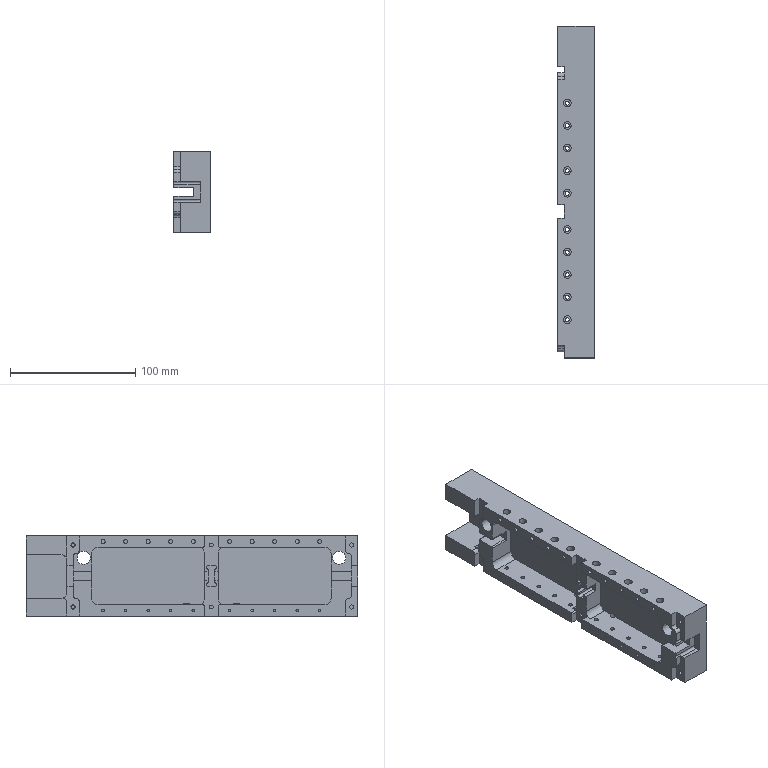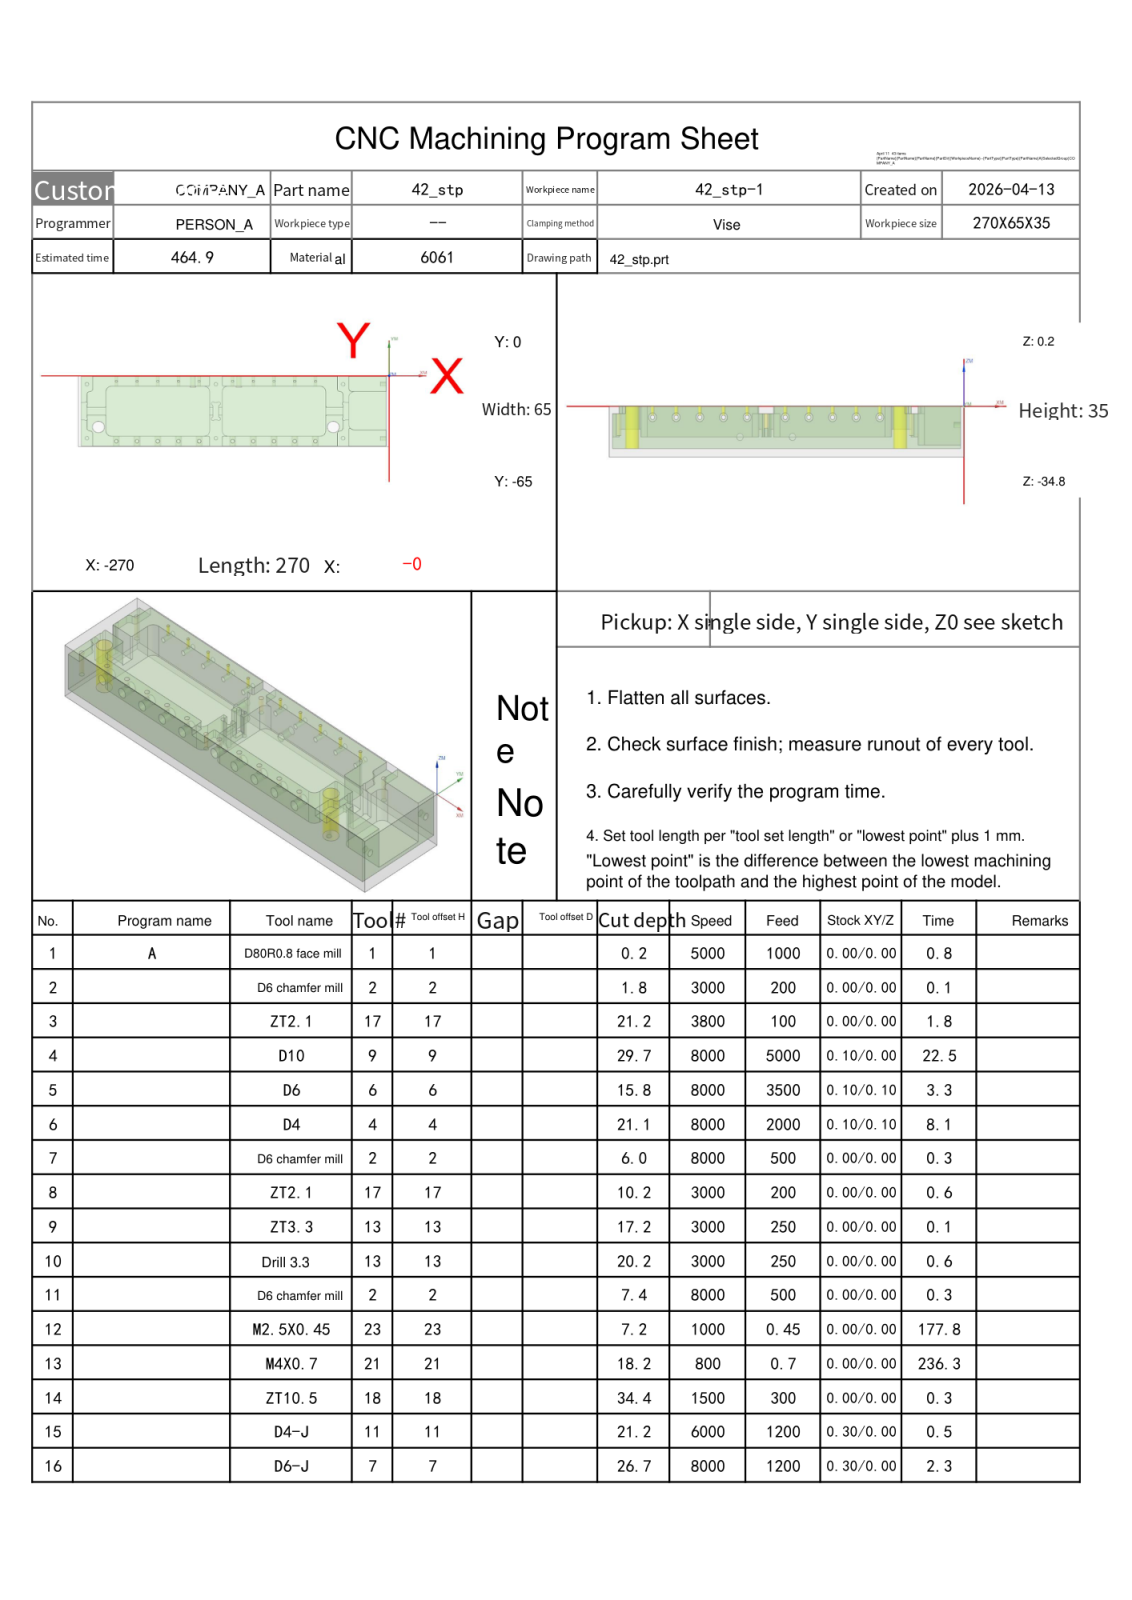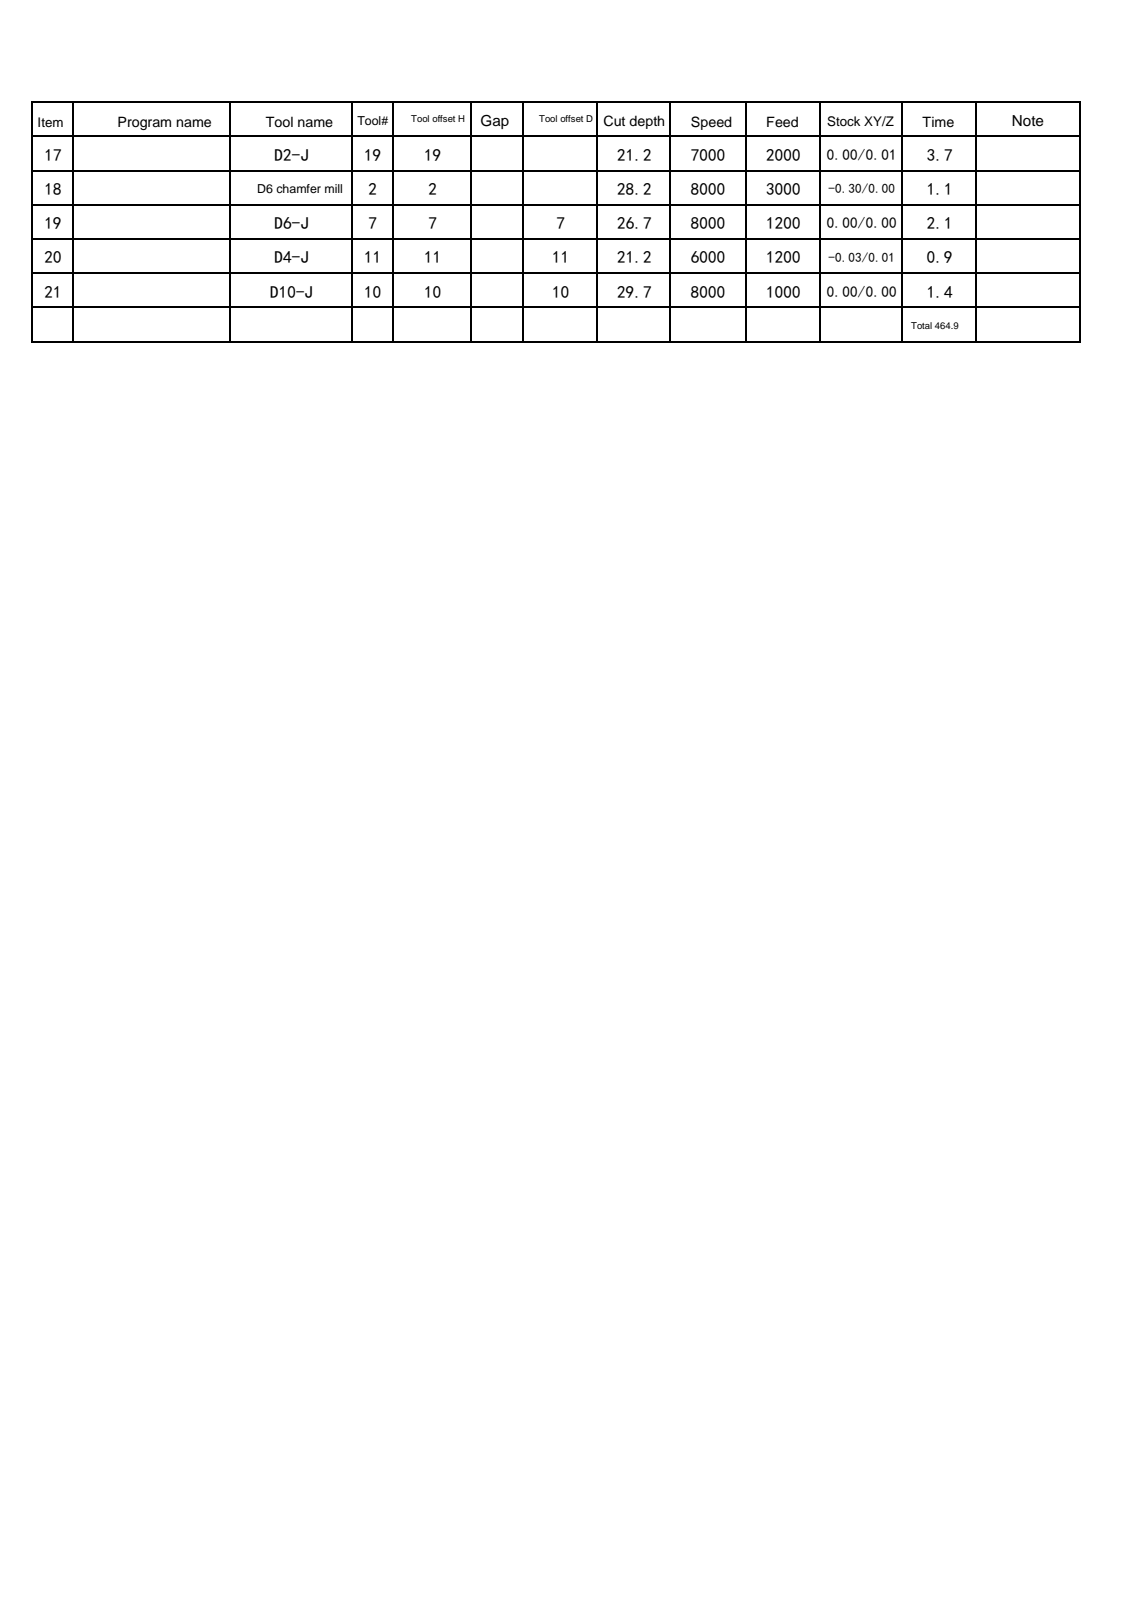NC program | NX | posted by the shop | part box 29 x 265 x 64 mm
Lines 1 to 4065 of 41846, first 2576 of 4063 lines:
%
O0001
(Machine time: 837.83 MIN)
(===Total Tool:14===)
(T1=D80R0.8 face mill D=80.  R=0.8  D-  H01 Z=-0.   )
(T2=D6 chamfer mill   D=6.   R=0.   D-  H02 Z=-28.  )
(T17=ZT2.1  D=2.1  DR_a=118 D-  H17 Z=-21.  )
(T9=D10     D=10.  R=0.   D-  H09 Z=-29.5 )
(T6=D6      D=6.   R=0.   D-  H06 Z=-15.6 )
(T4=D4      D=4.   R=0.   D-  H04 Z=-20.9 )
(T13=ZT3.3  D=3.3  DR_a=118 D-  H13 Z=-20.  )
(T23=M2.5X0.45 D=2.05 DR_a=180 D-  H23 Z=-7.   )
(T21=M4X0.7 D=3.3  DR_a=180 D-  H21 Z=-18.  )
(T18=ZT10.5 D=10.5 DR_a=118 D-  H18 Z=-34.15)
(T11=D4-J   D=4.   R=0.   D-  H11 Z=-21.  )
(T7=D6-J    D=6.   R=0.   D-  H07 Z=-26.5 )
(T19=D2-J   D=2.   R=0.   D-  H19 Z=-21.  )
(T10=D10-J  D=10.  R=0.   D10 H10 Z=-29.5 )
G80 G90 G17 G49 G40
G91 G28 Z0
M01
N1 T01 M06
(D80R0.8 face mill  D=80. R=0.8 H=01 ce=0.00 di=0.00)
G00 G90 G54 X-312.5 Y-8.5 M03 S5000
G43 H01 Z20.
M08
Z2.
G01 Z0.0 F1000.
X-307.5
X37.5
Y-56.5
X-307.5
X-312.5
Z2.
G00 Z20.
G91 G28 Z0.0
M05
M09
G91 G28 Z0.0
M01
N2 T02 M06
(D6 chamfer mill  D=6. R=0. H=02 ce=0.00 di=0.00)
G00 G90 G54 X-263.5 Y-25.5 M03 S3000
G43 H02 Z20.
M08
G98 G81 X-263.5 Y-25.5 Z-1.55 R1. F200.
Y-39.5
X-153. Y-25.5
Y-39.5
X-148. Y-25.5
Y-39.5
X-39. Y-25.5
Y-39.5
G80
G00 Z20.
G91 G28 Z0.0
M05
M09
G91 G28 Z0.0
M01
N3 T17 M06
(ZT2.1 D=2.1 DR_a=118 H=17)
G00 G90 G54 X-263.5 Y-25.5 M03 S3800
G43 H17 Z20.
M08
G98 G83 X-263.5 Y-25.5 Z-21. R1. F100. Q1.5
Y-39.5
X-153. Y-25.5
Y-39.5
X-148. Y-25.5
Y-39.5
X-39. Y-25.5
Y-39.5
G80
G00 Z20.
G91 G28 Z0.0
M05
M09
G91 G28 Z0.0
M01
N4 T09 M06
(D10  D=10. R=0. H=09 ce=0.10 di=0.00)
G00 G90 G54 X-135. Y-69.6 M03 S8000
G43 H09 Z20.
M08
Z.5
G01 X-267.5 Z.348 F5000.
G02 X-272.6 Y-64.5 Z.339 I0.0 J5.1
G01 Y-.5 Z.266
G02 X-267.5 Y4.6 Z.257 I5.1 J0.0
G01 X-2.5 Z-.046
G02 X2.6 Y-.5 Z-.055 I0.0 J-5.1
G01 Y-64.5 Z-.129
G02 X-2.5 Y-69.6 Z-.138 I-5.1 J0.0
G01 X-267.5 Z-.441
G02 X-272.6 Y-64.5 Z-.45 I0.0 J5.1
G01 Y-.5 Z-.523
G02 X-267.5 Y4.6 Z-.533 I5.1 J0.0
G01 X-2.5 Z-.836
G02 X2.6 Y-.5 Z-.845 I0.0 J-5.1
G01 Y-64.5 Z-.918
G02 X-2.5 Y-69.6 Z-.927 I-5.1 J0.0
G01 X-267.5 Z-1.231
G02 X-272.6 Y-64.5 Z-1.24 I0.0 J5.1
G01 Y-.5 Z-1.313
G02 X-267.5 Y4.6 Z-1.322 I5.1 J0.0
G01 X-2.5 Z-1.625
G02 X2.6 Y-.5 Z-1.634 I0.0 J-5.1
G01 Y-64.5 Z-1.708
G02 X-2.5 Y-69.6 Z-1.717 I-5.1 J0.0
G01 X-267.5 Z-2.02
G02 X-272.6 Y-64.5 Z-2.029 I0.0 J5.1
G01 Y-.5 Z-2.102
G02 X-267.5 Y4.6 Z-2.112 I5.1 J0.0
G01 X-2.5 Z-2.415
G02 X2.6 Y-.5 Z-2.424 I0.0 J-5.1
G01 Y-64.5 Z-2.497
G02 X-2.5 Y-69.6 Z-2.506 I-5.1 J0.0
G01 X-267.5 Z-2.809
G02 X-272.6 Y-64.5 Z-2.819 I0.0 J5.1
G01 Y-.5 Z-2.892
G02 X-267.5 Y4.6 Z-2.901 I5.1 J0.0
G01 X-2.5 Z-3.204
G02 X2.6 Y-.5 Z-3.213 I0.0 J-5.1
G01 Y-64.5 Z-3.287
G02 X-2.5 Y-69.6 Z-3.296 I-5.1 J0.0
G01 X-267.5 Z-3.599
G02 X-272.6 Y-64.5 Z-3.608 I0.0 J5.1
G01 Y-.5 Z-3.681
G02 X-267.5 Y4.6 Z-3.691 I5.1 J0.0
G01 X-2.5 Z-3.994
G02 X2.6 Y-.5 Z-4.003 I0.0 J-5.1
G01 Y-64.5 Z-4.076
G02 X-2.5 Y-69.6 Z-4.085 I-5.1 J0.0
G01 X-267.5 Z-4.388
G02 X-272.6 Y-64.5 Z-4.398 I0.0 J5.1
G01 Y-.5 Z-4.471
G02 X-267.5 Y4.6 Z-4.48 I5.1 J0.0
G01 X-2.5 Z-4.783
G02 X2.6 Y-.5 Z-4.792 I0.0 J-5.1
G01 Y-64.5 Z-4.866
G02 X-2.5 Y-69.6 Z-4.875 I-5.1 J0.0
G01 X-267.5 Z-5.178
G02 X-272.6 Y-64.5 Z-5.187 I0.0 J5.1
G01 Y-.5 Z-5.26
G02 X-267.5 Y4.6 Z-5.269 I5.1 J0.0
G01 X-2.5 Z-5.573
G02 X2.6 Y-.5 Z-5.582 I0.0 J-5.1
G01 Y-64.5 Z-5.655
G02 X-2.5 Y-69.6 Z-5.664 I-5.1 J0.0
G01 X-267.5 Z-5.967
G02 X-272.6 Y-64.5 Z-5.977 I0.0 J5.1
G01 Y-.5 Z-6.05
G02 X-267.5 Y4.6 Z-6.059 I5.1 J0.0
G01 X-2.5 Z-6.362
G02 X2.6 Y-.5 Z-6.371 I0.0 J-5.1
G01 Y-64.5 Z-6.445
G02 X-2.5 Y-69.6 Z-6.454 I-5.1 J0.0
G01 X-267.5 Z-6.757
G02 X-272.6 Y-64.5 Z-6.766 I0.0 J5.1
G01 Y-.5 Z-6.839
G02 X-267.5 Y4.6 Z-6.848 I5.1 J0.0
G01 X-2.5 Z-7.152
G02 X2.6 Y-.5 Z-7.161 I0.0 J-5.1
G01 Y-64.5 Z-7.234
G02 X-2.5 Y-69.6 Z-7.243 I-5.1 J0.0
G01 X-267.5 Z-7.546
G02 X-272.6 Y-64.5 Z-7.555 I0.0 J5.1
G01 Y-.5 Z-7.629
G02 X-267.5 Y4.6 Z-7.638 I5.1 J0.0
G01 X-2.5 Z-7.941
G02 X2.6 Y-.5 Z-7.95 I0.0 J-5.1
G01 Y-64.5 Z-8.023
G02 X-2.5 Y-69.6 Z-8.033 I-5.1 J0.0
G01 X-267.5 Z-8.336
G02 X-272.6 Y-64.5 Z-8.345 I0.0 J5.1
G01 Y-.5 Z-8.418
G02 X-267.5 Y4.6 Z-8.427 I5.1 J0.0
G01 X-2.5 Z-8.731
G02 X2.6 Y-.5 Z-8.74 I0.0 J-5.1
G01 Y-64.5 Z-8.813
G02 X-2.5 Y-69.6 Z-8.822 I-5.1 J0.0
G01 X-267.5 Z-9.125
G02 X-272.6 Y-64.5 Z-9.134 I0.0 J5.1
G01 Y-.5 Z-9.208
G02 X-267.5 Y4.6 Z-9.217 I5.1 J0.0
G01 X-2.5 Z-9.52
G02 X2.6 Y-.5 Z-9.529 I0.0 J-5.1
G01 Y-64.5 Z-9.602
G02 X-2.5 Y-69.6 Z-9.612 I-5.1 J0.0
G01 X-267.5 Z-9.915
G02 X-272.6 Y-64.5 Z-9.924 I0.0 J5.1
G01 Y-.5 Z-9.997
G02 X-267.5 Y4.6 Z-10.006 I5.1 J0.0
G01 X-2.5 Z-10.309
G02 X2.6 Y-.5 Z-10.319 I0.0 J-5.1
G01 Y-64.5 Z-10.392
G02 X-2.5 Y-69.6 Z-10.401 I-5.1 J0.0
G01 X-267.5 Z-10.704
G02 X-272.6 Y-64.5 Z-10.713 I0.0 J5.1
G01 Y-.5 Z-10.787
G02 X-267.5 Y4.6 Z-10.796 I5.1 J0.0
G01 X-2.5 Z-11.099
G02 X2.6 Y-.5 Z-11.108 I0.0 J-5.1
G01 Y-64.5 Z-11.181
G02 X-2.5 Y-69.6 Z-11.191 I-5.1 J0.0
G01 X-267.5 Z-11.494
G02 X-272.6 Y-64.5 Z-11.503 I0.0 J5.1
G01 Y-.5 Z-11.576
G02 X-267.5 Y4.6 Z-11.585 I5.1 J0.0
G01 X-2.5 Z-11.888
G02 X2.6 Y-.5 Z-11.898 I0.0 J-5.1
G01 Y-64.5 Z-11.971
G02 X-2.5 Y-69.6 Z-11.98 I-5.1 J0.0
G01 X-267.5 Z-12.283
G02 X-272.6 Y-64.5 Z-12.292 I0.0 J5.1
G01 Y-.5 Z-12.366
G02 X-267.5 Y4.6 Z-12.375 I5.1 J0.0
G01 X-2.5 Z-12.678
G02 X2.6 Y-.5 Z-12.687 I0.0 J-5.1
G01 Y-64.5 Z-12.76
G02 X-2.5 Y-69.6 Z-12.769 I-5.1 J0.0
G01 X-267.5 Z-13.073
G02 X-272.6 Y-64.5 Z-13.082 I0.0 J5.1
G01 Y-.5 Z-13.155
G02 X-267.5 Y4.6 Z-13.164 I5.1 J0.0
G01 X-2.5 Z-13.467
G02 X2.6 Y-.5 Z-13.477 I0.0 J-5.1
G01 Y-64.5 Z-13.55
G02 X-2.5 Y-69.6 Z-13.559 I-5.1 J0.0
G01 X-267.5 Z-13.862
G02 X-272.6 Y-64.5 Z-13.871 I0.0 J5.1
G01 Y-.5 Z-13.945
G02 X-267.5 Y4.6 Z-13.954 I5.1 J0.0
G01 X-2.5 Z-14.257
G02 X2.6 Y-.5 Z-14.266 I0.0 J-5.1
G01 Y-64.5 Z-14.339
G02 X-2.5 Y-69.6 Z-14.348 I-5.1 J0.0
G01 X-267.5 Z-14.652
G02 X-272.6 Y-64.5 Z-14.661 I0.0 J5.1
G01 Y-.5 Z-14.734
G02 X-267.5 Y4.6 Z-14.743 I5.1 J0.0
G01 X-2.5 Z-15.046
G02 X2.6 Y-.5 Z-15.055 I0.0 J-5.1
G01 Y-64.5 Z-15.129
G02 X-2.5 Y-69.6 Z-15.138 I-5.1 J0.0
G01 X-267.5 Z-15.441
G02 X-272.6 Y-64.5 Z-15.45 I0.0 J5.1
G01 Y-.5 Z-15.523
G02 X-267.5 Y4.6 Z-15.533 I5.1 J0.0
G01 X-2.5 Z-15.836
G02 X2.6 Y-.5 Z-15.845 I0.0 J-5.1
G01 Y-64.5 Z-15.918
G02 X-2.5 Y-69.6 Z-15.927 I-5.1 J0.0
G01 X-267.5 Z-16.231
G02 X-272.6 Y-64.5 Z-16.24 I0.0 J5.1
G01 Y-.5 Z-16.313
G02 X-267.5 Y4.6 Z-16.322 I5.1 J0.0
G01 X-2.5 Z-16.625
G02 X2.6 Y-.5 Z-16.634 I0.0 J-5.1
G01 Y-64.5 Z-16.708
G02 X-2.5 Y-69.6 Z-16.717 I-5.1 J0.0
G01 X-267.5 Z-17.02
G02 X-272.6 Y-64.5 Z-17.029 I0.0 J5.1
G01 Y-.5 Z-17.102
G02 X-267.5 Y4.6 Z-17.112 I5.1 J0.0
G01 X-2.5 Z-17.415
G02 X2.6 Y-.5 Z-17.424 I0.0 J-5.1
G01 Y-64.5 Z-17.497
G02 X-2.5 Y-69.6 Z-17.506 I-5.1 J0.0
G01 X-267.5 Z-17.809
G02 X-272.6 Y-64.5 Z-17.819 I0.0 J5.1
G01 Y-.5 Z-17.892
G02 X-267.5 Y4.6 Z-17.901 I5.1 J0.0
G01 X-2.5 Z-18.204
G02 X2.6 Y-.5 Z-18.213 I0.0 J-5.1
G01 Y-64.5 Z-18.287
G02 X-2.5 Y-69.6 Z-18.296 I-5.1 J0.0
G01 X-267.5 Z-18.599
G02 X-272.6 Y-64.5 Z-18.608 I0.0 J5.1
G01 Y-.5 Z-18.681
G02 X-267.5 Y4.6 Z-18.691 I5.1 J0.0
G01 X-2.5 Z-18.994
G02 X2.6 Y-.5 Z-19.003 I0.0 J-5.1
G01 Y-64.5 Z-19.076
G02 X-2.5 Y-69.6 Z-19.085 I-5.1 J0.0
G01 X-267.5 Z-19.388
G02 X-272.6 Y-64.5 Z-19.398 I0.0 J5.1
G01 Y-.5 Z-19.471
G02 X-267.5 Y4.6 Z-19.48 I5.1 J0.0
G01 X-2.5 Z-19.783
G02 X2.6 Y-.5 Z-19.792 I0.0 J-5.1
G01 Y-64.5 Z-19.866
G02 X-2.5 Y-69.6 Z-19.875 I-5.1 J0.0
G01 X-267.5 Z-20.178
G02 X-272.6 Y-64.5 Z-20.187 I0.0 J5.1
G01 Y-.5 Z-20.26
G02 X-267.5 Y4.6 Z-20.269 I5.1 J0.0
G01 X-2.5 Z-20.573
G02 X2.6 Y-.5 Z-20.582 I0.0 J-5.1
G01 Y-64.5 Z-20.655
G02 X-2.5 Y-69.6 Z-20.664 I-5.1 J0.0
G01 X-267.5 Z-20.967
G02 X-272.6 Y-64.5 Z-20.977 I0.0 J5.1
G01 Y-.5 Z-21.05
G02 X-267.5 Y4.6 Z-21.059 I5.1 J0.0
G01 X-2.5 Z-21.362
G02 X2.6 Y-.5 Z-21.371 I0.0 J-5.1
G01 Y-64.5 Z-21.445
G02 X-2.5 Y-69.6 Z-21.454 I-5.1 J0.0
G01 X-267.5 Z-21.757
G02 X-272.6 Y-64.5 Z-21.766 I0.0 J5.1
G01 Y-.5 Z-21.839
G02 X-267.5 Y4.6 Z-21.848 I5.1 J0.0
G01 X-2.5 Z-22.152
G02 X2.6 Y-.5 Z-22.161 I0.0 J-5.1
G01 Y-64.5 Z-22.234
G02 X-2.5 Y-69.6 Z-22.243 I-5.1 J0.0
G01 X-267.5 Z-22.546
G02 X-272.6 Y-64.5 Z-22.555 I0.0 J5.1
G01 Y-.5 Z-22.629
G02 X-267.5 Y4.6 Z-22.638 I5.1 J0.0
G01 X-2.5 Z-22.941
G02 X2.6 Y-.5 Z-22.95 I0.0 J-5.1
G01 Y-64.5 Z-23.023
G02 X-2.5 Y-69.6 Z-23.033 I-5.1 J0.0
G01 X-267.5 Z-23.336
G02 X-272.6 Y-64.5 Z-23.345 I0.0 J5.1
G01 Y-.5 Z-23.418
G02 X-267.5 Y4.6 Z-23.427 I5.1 J0.0
G01 X-2.5 Z-23.731
G02 X2.6 Y-.5 Z-23.74 I0.0 J-5.1
G01 Y-64.5 Z-23.813
G02 X-2.5 Y-69.6 Z-23.822 I-5.1 J0.0
G01 X-267.5 Z-24.125
G02 X-272.6 Y-64.5 Z-24.134 I0.0 J5.1
G01 Y-.5 Z-24.208
G02 X-267.5 Y4.6 Z-24.217 I5.1 J0.0
G01 X-2.5 Z-24.52
G02 X2.6 Y-.5 Z-24.529 I0.0 J-5.1
G01 Y-64.5 Z-24.602
G02 X-2.5 Y-69.6 Z-24.612 I-5.1 J0.0
G01 X-267.5 Z-24.915
G02 X-272.6 Y-64.5 Z-24.924 I0.0 J5.1
G01 Y-.5 Z-24.997
G02 X-267.5 Y4.6 Z-25.006 I5.1 J0.0
G01 X-2.5 Z-25.309
G02 X2.6 Y-.5 Z-25.319 I0.0 J-5.1
G01 Y-64.5 Z-25.392
G02 X-2.5 Y-69.6 Z-25.401 I-5.1 J0.0
G01 X-267.5 Z-25.704
G02 X-272.6 Y-64.5 Z-25.713 I0.0 J5.1
G01 Y-.5 Z-25.787
G02 X-267.5 Y4.6 Z-25.796 I5.1 J0.0
G01 X-2.5 Z-26.099
G02 X2.6 Y-.5 Z-26.108 I0.0 J-5.1
G01 Y-64.5 Z-26.181
G02 X-2.5 Y-69.6 Z-26.191 I-5.1 J0.0
G01 X-267.5 Z-26.494
G02 X-272.6 Y-64.5 Z-26.503 I0.0 J5.1
G01 Y-.5 Z-26.576
G02 X-267.5 Y4.6 Z-26.585 I5.1 J0.0
G01 X-2.5 Z-26.888
G02 X2.6 Y-.5 Z-26.898 I0.0 J-5.1
G01 Y-64.5 Z-26.971
G02 X-2.5 Y-69.6 Z-26.98 I-5.1 J0.0
G01 X-267.5 Z-27.283
G02 X-272.6 Y-64.5 Z-27.292 I0.0 J5.1
G01 Y-.5 Z-27.366
G02 X-267.5 Y4.6 Z-27.375 I5.1 J0.0
G01 X-2.5 Z-27.678
G02 X2.6 Y-.5 Z-27.687 I0.0 J-5.1
G01 Y-64.5 Z-27.76
G02 X-2.5 Y-69.6 Z-27.769 I-5.1 J0.0
G01 X-267.5 Z-28.073
G02 X-272.6 Y-64.5 Z-28.082 I0.0 J5.1
G01 Y-.5 Z-28.155
G02 X-267.5 Y4.6 Z-28.164 I5.1 J0.0
G01 X-2.5 Z-28.467
G02 X2.6 Y-.5 Z-28.477 I0.0 J-5.1
G01 Y-64.5 Z-28.55
G02 X-2.5 Y-69.6 Z-28.559 I-5.1 J0.0
G01 X-267.5 Z-28.862
G02 X-272.6 Y-64.5 Z-28.871 I0.0 J5.1
G01 Y-.5 Z-28.945
G02 X-267.5 Y4.6 Z-28.954 I5.1 J0.0
G01 X-2.5 Z-29.257
G02 X2.6 Y-.5 Z-29.266 I0.0 J-5.1
G01 Y-64.5 Z-29.339
G02 X-2.5 Y-69.6 Z-29.348 I-5.1 J0.0
G01 X-135. Z-29.5
X-267.5
G02 X-272.6 Y-64.5 I0.0 J5.1
G01 Y-.5
G02 X-267.5 Y4.6 I5.1 J0.0
G01 X-2.5
G02 X2.6 Y-.5 I0.0 J-5.1
G01 Y-64.5
G02 X-2.5 Y-69.6 I-5.1 J0.0
G01 X-135.
X-135.5
Z-28.5
G00 Z20.
G00 G90 X-179.498 Y-36.4 M03 S8000
Z20.
Z.5
G01 X-175.1 Z.385 F3500.
Y-28.6 Z.181
X-201. Z-.498
X-226.9
Y-36.4
X-175.1
Y-28.6
X-201.
Y-21.6
X-233.9
Y-43.4
X-168.1
Y-21.6
X-201.
Y-14.6
X-240.9
Y-50.4
X-161.1
Y-14.6
X-201.
X-201.5
Z.002
G00 Z.5
X-179.498 Y-36.4
Z.002
G01 X-175.1 Z-.113
Y-28.6 Z-.317
X-201. Z-.995
X-226.9
Y-36.4
X-175.1
Y-28.6
X-201.
Y-21.6
X-233.9
Y-43.4
X-168.1
Y-21.6
X-201.
Y-14.6
X-240.9
Y-50.4
X-161.1
Y-14.6
X-201.
X-201.5
Z-.495
G00 Z.002
X-179.498 Y-36.4
Z-.495
G01 X-175.1 Z-.61
Y-28.6 Z-.815
X-201. Z-1.493
X-226.9
Y-36.4
X-175.1
Y-28.6
X-201.
Y-21.6
X-233.9
Y-43.4
X-168.1
Y-21.6
X-201.
Y-14.6
X-240.9
Y-50.4
X-161.1
Y-14.6
X-201.
X-201.5
Z-.993
G00 Z-.495
X-179.498 Y-36.4
Z-.993
G01 X-175.1 Z-1.108
Y-28.6 Z-1.312
X-201. Z-1.99
X-226.9
Y-36.4
X-175.1
Y-28.6
X-201.
Y-21.6
X-233.9
Y-43.4
X-168.1
Y-21.6
X-201.
Y-14.6
X-240.9
Y-50.4
X-161.1
Y-14.6
X-201.
X-201.5
Z-1.49
G00 Z-.993
X-179.498 Y-36.4
Z-1.49
G01 X-175.1 Z-1.606
Y-28.6 Z-1.81
X-201. Z-2.488
X-226.9
Y-36.4
X-175.1
Y-28.6
X-201.
Y-21.6
X-233.9
Y-43.4
X-168.1
Y-21.6
X-201.
Y-14.6
X-240.9
Y-50.4
X-161.1
Y-14.6
X-201.
X-201.5
Z-1.988
G00 Z-1.49
X-179.498 Y-36.4
Z-1.988
G01 X-175.1 Z-2.103
Y-28.6 Z-2.307
X-201. Z-2.986
X-226.9
Y-36.4
X-175.1
Y-28.6
X-201.
Y-21.6
X-233.9
Y-43.4
X-168.1
Y-21.6
X-201.
Y-14.6
X-240.9
Y-50.4
X-161.1
Y-14.6
X-201.
X-201.5
Z-2.486
G00 Z-1.988
X-179.498 Y-36.4
Z-2.486
G01 X-175.1 Z-2.601
Y-28.6 Z-2.805
X-201. Z-3.483
X-226.9
Y-36.4
X-175.1
Y-28.6
X-201.
Y-21.6
X-233.9
Y-43.4
X-168.1
Y-21.6
X-201.
Y-14.6
X-240.9
Y-50.4
X-161.1
Y-14.6
X-201.
X-201.5
Z-2.983
G00 Z-2.486
X-179.498 Y-36.4
Z-2.983
G01 X-175.1 Z-3.098
Y-28.6 Z-3.303
X-201. Z-3.981
X-226.9
Y-36.4
X-175.1
Y-28.6
X-201.
Y-21.6
X-233.9
Y-43.4
X-168.1
Y-21.6
X-201.
Y-14.6
X-240.9
Y-50.4
X-161.1
Y-14.6
X-201.
X-201.5
Z-3.481
G00 Z-2.983
X-179.498 Y-36.4
Z-3.481
G01 X-175.1 Z-3.596
Y-28.6 Z-3.8
X-201. Z-4.479
X-226.9
Y-36.4
X-175.1
Y-28.6
X-201.
Y-21.6
X-233.9
Y-43.4
X-168.1
Y-21.6
X-201.
Y-14.6
X-240.9
Y-50.4
X-161.1
Y-14.6
X-201.
X-201.5
Z-3.979
G00 Z-3.481
X-179.498 Y-36.4
Z-3.979
G01 X-175.1 Z-4.094
Y-28.6 Z-4.298
X-201. Z-4.976
X-226.9
Y-36.4
X-175.1
Y-28.6
X-201.
Y-21.6
X-233.9
Y-43.4
X-168.1
Y-21.6
X-201.
Y-14.6
X-240.9
Y-50.4
X-161.1
Y-14.6
X-201.
X-201.5
Z-4.476
G00 Z-3.979
X-179.498 Y-36.4
Z-4.476
G01 X-175.1 Z-4.591
Y-28.6 Z-4.796
X-201. Z-5.474
X-226.9
Y-36.4
X-175.1
Y-28.6
X-201.
Y-21.6
X-233.9
Y-43.4
X-168.1
Y-21.6
X-201.
Y-14.6
X-240.9
Y-50.4
X-161.1
Y-14.6
X-201.
X-201.5
Z-4.974
G00 Z-4.476
X-179.498 Y-36.4
Z-4.974
G01 X-175.1 Z-5.089
Y-28.6 Z-5.293
X-201. Z-5.971
X-226.9
Y-36.4
X-175.1
Y-28.6
X-201.
Y-21.6
X-233.9
Y-43.4
X-168.1
Y-21.6
X-201.
Y-14.6
X-240.9
Y-50.4
X-161.1
Y-14.6
X-201.
X-201.5
Z-5.471
G00 Z-4.974
X-179.498 Y-36.4
Z-5.471
G01 X-175.1 Z-5.587
Y-28.6 Z-5.791
X-201. Z-6.469
X-226.9
Y-36.4
X-175.1
Y-28.6
X-201.
Y-21.6
X-233.9
Y-43.4
X-168.1
Y-21.6
X-201.
Y-14.6
X-240.9
Y-50.4
X-161.1
Y-14.6
X-201.
X-201.5
Z-5.969
G00 Z-5.471
X-179.498 Y-36.4
Z-5.969
G01 X-175.1 Z-6.084
Y-28.6 Z-6.288
X-201. Z-6.967
X-226.9
Y-36.4
X-175.1
Y-28.6
X-201.
Y-21.6
X-233.9
Y-43.4
X-168.1
Y-21.6
X-201.
Y-14.6
X-240.9
Y-50.4
X-161.1
Y-14.6
X-201.
X-201.5
Z-6.467
G00 Z-5.969
X-179.498 Y-36.4
Z-6.467
G01 X-175.1 Z-6.582
Y-28.6 Z-6.786
X-201. Z-7.464
X-226.9
Y-36.4
X-175.1
Y-28.6
X-201.
Y-21.6
X-233.9
Y-43.4
X-168.1
Y-21.6
X-201.
Y-14.6
X-240.9
Y-50.4
X-161.1
Y-14.6
X-201.
X-201.5
Z-6.964
G00 Z-6.467
X-179.498 Y-36.4
Z-6.964
G01 X-175.1 Z-7.079
Y-28.6 Z-7.284
X-201. Z-7.962
X-226.9
Y-36.4
X-175.1
Y-28.6
X-201.
Y-21.6
X-233.9
Y-43.4
X-168.1
Y-21.6
X-201.
Y-14.6
X-240.9
Y-50.4
X-161.1
Y-14.6
X-201.
X-201.5
Z-7.462
G00 Z-6.964
X-179.498 Y-36.4
Z-7.462
G01 X-175.1 Z-7.577
Y-28.6 Z-7.781
X-201. Z-8.46
X-226.9
Y-36.4
X-175.1
Y-28.6
X-201.
Y-21.6
X-233.9
Y-43.4
X-168.1
Y-21.6
X-201.
Y-14.6
X-240.9
Y-50.4
X-161.1
Y-14.6
X-201.
X-201.5
Z-7.96
G00 Z-7.462
X-179.498 Y-36.4
Z-7.96
G01 X-175.1 Z-8.075
Y-28.6 Z-8.279
X-201. Z-8.957
X-226.9
Y-36.4
X-175.1
Y-28.6
X-201.
Y-21.6
X-233.9
Y-43.4
X-168.1
Y-21.6
X-201.
Y-14.6
X-240.9
Y-50.4
X-161.1
Y-14.6
X-201.
X-201.5
Z-8.457
G00 Z-7.96
X-179.498 Y-36.4
Z-8.457
G01 X-175.1 Z-8.572
Y-28.6 Z-8.777
X-201. Z-9.455
X-226.9
Y-36.4
X-175.1
Y-28.6
X-201.
Y-21.6
X-233.9
Y-43.4
X-168.1
Y-21.6
X-201.
Y-14.6
X-240.9
Y-50.4
X-161.1
Y-14.6
X-201.
X-201.5
Z-8.955
G00 Z-8.457
X-179.498 Y-36.4
Z-8.955
G01 X-175.1 Z-9.07
Y-28.6 Z-9.274
X-201. Z-9.952
X-226.9
Y-36.4
X-175.1
Y-28.6
X-201.
Y-21.6
X-233.9
Y-43.4
X-168.1
Y-21.6
X-201.
Y-14.6
X-240.9
Y-50.4
X-161.1
Y-14.6
X-201.
X-201.5
Z-9.452
G00 Z-8.955
X-179.498 Y-36.4
Z-9.452
G01 X-175.1 Z-9.568
Y-28.6 Z-9.772
X-201. Z-10.45
X-226.9
Y-36.4
X-175.1
Y-28.6
X-201.
Y-21.6
X-233.9
Y-43.4
X-168.1
Y-21.6
X-201.
Y-14.6
X-240.9
Y-50.4
X-161.1
Y-14.6
X-201.
X-201.5
Z-9.95
G00 Z-9.452
X-179.498 Y-36.4
Z-9.95
G01 X-175.1 Z-10.065
Y-28.6 Z-10.269
X-201. Z-10.948
X-226.9
Y-36.4
X-175.1
Y-28.6
X-201.
Y-21.6
X-233.9
Y-43.4
X-168.1
Y-21.6
X-201.
Y-14.6
X-240.9
Y-50.4
X-161.1
Y-14.6
X-201.
X-201.5
Z-10.448
G00 Z-9.95
X-179.498 Y-36.4
Z-10.448
G01 X-175.1 Z-10.563
Y-28.6 Z-10.767
X-201. Z-11.445
X-226.9
Y-36.4
X-175.1
Y-28.6
X-201.
Y-21.6
X-233.9
Y-43.4
X-168.1
Y-21.6
X-201.
Y-14.6
X-240.9
Y-50.4
X-161.1
Y-14.6
X-201.
X-201.5
Z-10.945
G00 Z-10.448
X-179.498 Y-36.4
Z-10.945
G01 X-175.1 Z-11.06
Y-28.6 Z-11.265
X-201. Z-11.943
X-226.9
Y-36.4
X-175.1
Y-28.6
X-201.
Y-21.6
X-233.9
Y-43.4
X-168.1
Y-21.6
X-201.
Y-14.6
X-240.9
Y-50.4
X-161.1
Y-14.6
X-201.
X-201.5
Z-11.443
G00 Z-10.945
X-179.498 Y-36.4
Z-11.443
G01 X-175.1 Z-11.558
Y-28.6 Z-11.762
X-201. Z-12.44
X-226.9
Y-36.4
X-175.1
Y-28.6
X-201.
Y-21.6
X-233.9
Y-43.4
X-168.1
Y-21.6
X-201.
Y-14.6
X-240.9
Y-50.4
X-161.1
Y-14.6
X-201.
X-201.5
Z-11.94
G00 Z-11.443
X-179.498 Y-36.4
Z-11.94
G01 X-175.1 Z-12.056
Y-28.6 Z-12.26
X-201. Z-12.938
X-226.9
Y-36.4
X-175.1
Y-28.6
X-201.
Y-21.6
X-233.9
Y-43.4
X-168.1
Y-21.6
X-201.
Y-14.6
X-240.9
Y-50.4
X-161.1
Y-14.6
X-201.
X-201.5
Z-12.438
G00 Z-11.94
X-179.498 Y-36.4
Z-12.438
G01 X-175.1 Z-12.553
Y-28.6 Z-12.757
X-201. Z-13.436
X-226.9
Y-36.4
X-175.1
Y-28.6
X-201.
Y-21.6
X-233.9
Y-43.4
X-168.1
Y-21.6
X-201.
Y-14.6
X-240.9
Y-50.4
X-161.1
Y-14.6
X-201.
X-201.5
Z-12.936
G00 Z-12.438
X-179.498 Y-36.4
Z-12.936
G01 X-175.1 Z-13.051
Y-28.6 Z-13.255
X-201. Z-13.933
X-226.9
Y-36.4
X-175.1
Y-28.6
X-201.
Y-21.6
X-233.9
Y-43.4
X-168.1
Y-21.6
X-201.
Y-14.6
X-240.9
Y-50.4
X-161.1
Y-14.6
X-201.
X-201.5
Z-13.433
G00 Z-12.936
X-179.498 Y-36.4
Z-13.433
G01 X-175.1 Z-13.548
Y-28.6 Z-13.753
X-201. Z-14.431
X-226.9
Y-36.4
X-175.1
Y-28.6
X-201.
Y-21.6
X-233.9
Y-43.4
X-168.1
Y-21.6
X-201.
Y-14.6
X-240.9
Y-50.4
X-161.1
Y-14.6
X-201.
X-201.5
Z-13.931
G00 Z-13.433
X-179.498 Y-36.4
Z-13.931
G01 X-175.1 Z-14.046
Y-28.6 Z-14.25
X-201. Z-14.929
X-226.9
Y-36.4
X-175.1
Y-28.6
X-201.
Y-21.6
X-233.9
Y-43.4
X-168.1
Y-21.6
X-201.
Y-14.6
X-240.9
Y-50.4
X-161.1
Y-14.6
X-201.
X-201.5
Z-14.429
G00 Z-13.931
X-179.498 Y-36.4
Z-14.429
G01 X-175.1 Z-14.544
Y-28.6 Z-14.748
X-201. Z-15.426
X-226.9
Y-36.4
X-175.1
Y-28.6
X-201.
Y-21.6
X-233.9
Y-43.4
X-168.1
Y-21.6
X-201.
Y-14.6
X-240.9
Y-50.4
X-161.1
Y-14.6
X-201.
X-201.5
Z-14.926
G00 Z-14.429
X-179.498 Y-36.4
Z-14.926
G01 X-175.1 Z-15.041
Y-28.6 Z-15.246
X-201. Z-15.924
X-226.9
Y-36.4
X-175.1
Y-28.6
X-201.
Y-21.6
X-233.9
Y-43.4
X-168.1
Y-21.6
X-201.
Y-14.6
X-240.9
Y-50.4
X-161.1
Y-14.6
X-201.
X-201.5
Z-15.424
G00 Z-14.926
X-179.498 Y-36.4
Z-15.424
G01 X-175.1 Z-15.539
Y-28.6 Z-15.743
X-201. Z-16.421
X-226.9
Y-36.4
X-175.1
Y-28.6
X-201.
Y-21.6
X-233.9
Y-43.4
X-168.1
Y-21.6
X-201.
Y-14.6
X-240.9
Y-50.4
X-161.1
Y-14.6
X-201.
X-201.5
Z-15.921
G00 Z-15.424
X-179.498 Y-36.4
Z-15.921
G01 X-175.1 Z-16.037
Y-28.6 Z-16.241
X-201. Z-16.919
X-226.9
Y-36.4
X-175.1
Y-28.6
X-201.
Y-21.6
X-233.9
Y-43.4
X-168.1
Y-21.6
X-201.
Y-14.6
X-240.9
Y-50.4
X-161.1
Y-14.6
X-201.
X-201.5
Z-16.419
G00 Z-15.921
X-179.498 Y-36.4
Z-16.419
G01 X-175.1 Z-16.534
Y-28.6 Z-16.738
X-201. Z-17.417
X-226.9
Y-36.4
X-175.1
Y-28.6
X-201.
Y-21.6
X-233.9
Y-43.4
X-168.1
Y-21.6
X-201.
Y-14.6
X-240.9
Y-50.4
X-161.1
Y-14.6
X-201.
X-201.5
Z-16.917
G00 Z-16.419
X-179.498 Y-36.4
Z-16.917
G01 X-175.1 Z-17.032
Y-28.6 Z-17.236
X-201. Z-17.914
X-226.9
Y-36.4
X-175.1
Y-28.6
X-201.
Y-21.6
X-233.9
Y-43.4
X-168.1
Y-21.6
X-201.
Y-14.6
X-240.9
Y-50.4
X-161.1
Y-14.6
X-201.
X-201.5
Z-17.414
G00 Z-16.917
X-179.498 Y-36.4
Z-17.414
G01 X-175.1 Z-17.529
Y-28.6 Z-17.734
X-201. Z-18.412
X-226.9
Y-36.4
X-175.1
Y-28.6
X-201.
Y-21.6
X-233.9
Y-43.4
X-168.1
Y-21.6
X-201.
Y-14.6
X-240.9
Y-50.4
X-161.1
Y-14.6
X-201.
X-201.5
Z-17.912
G00 Z-17.414
X-179.498 Y-36.4
Z-17.912
G01 X-175.1 Z-18.027
Y-28.6 Z-18.231
X-201. Z-18.91
X-226.9
Y-36.4
X-175.1
Y-28.6
X-201.
Y-21.6
X-233.9
Y-43.4
X-168.1
Y-21.6
X-201.
Y-14.6
X-240.9
Y-50.4
X-161.1
Y-14.6
X-201.
X-201.5
Z-18.41
G00 Z-17.912
X-179.498 Y-36.4
Z-18.41
G01 X-175.1 Z-18.525
Y-28.6 Z-18.729
X-201. Z-19.407
X-226.9
Y-36.4
X-175.1
Y-28.6
X-201.
Y-21.6
X-233.9
Y-43.4
X-168.1
Y-21.6
X-201.
Y-14.6
X-240.9
Y-50.4
X-161.1
Y-14.6
X-201.
X-201.5
Z-18.907
G00 Z-18.41
X-179.498 Y-36.4
Z-18.907
G01 X-175.1 Z-19.022
Y-28.6 Z-19.227
X-201. Z-19.905
X-226.9
Y-36.4
X-175.1
Y-28.6
X-201.
Y-21.6
X-233.9
Y-43.4
X-168.1
Y-21.6
X-201.
Y-14.6
X-240.9
Y-50.4
X-161.1
Y-14.6
X-201.
X-201.5
Z-19.405
G00 Z-18.907
X-179.498 Y-36.4
Z-19.405
G01 X-175.1 Z-19.52
Y-28.6 Z-19.724
X-201. Z-20.402
X-226.9
Y-36.4
X-175.1
Y-28.6
X-201.
Y-21.6
X-233.9
Y-43.4
X-168.1
Y-21.6
X-201.
Y-14.6
X-240.9
Y-50.4
X-161.1
Y-14.6
X-201.
X-201.5
Z-19.902
G00 Z-19.405
X-179.498 Y-36.4
Z-19.902
G01 X-175.1 Z-20.018
Y-28.6 Z-20.222
X-201. Z-20.9
X-226.9
Y-36.4
X-175.1
Y-28.6
X-201.
Y-21.6
X-233.9
Y-43.4
X-168.1
Y-21.6
X-201.
Y-14.6
X-240.9
Y-50.4
X-161.1
Y-14.6
X-201.
X-201.5
Z-20.4
G00 Z20.
X-78.498 Y-36.4
Z.5
G01 X-74.1 Z.385
Y-28.6 Z.181
X-100. Z-.498
X-125.9
Y-36.4
X-74.1
Y-28.6
X-100.
Y-21.6
X-132.9
Y-43.4
X-67.1
Y-21.6
X-100.
Y-14.6
X-139.9
Y-50.4
X-60.1
Y-14.6
X-100.
X-100.5
Z.002
G00 Z.5
X-78.498 Y-36.4
Z.002
G01 X-74.1 Z-.113
Y-28.6 Z-.317
X-100. Z-.995
X-125.9
Y-36.4
X-74.1
Y-28.6
X-100.
Y-21.6
X-132.9
Y-43.4
X-67.1
Y-21.6
X-100.
Y-14.6
X-139.9
Y-50.4
X-60.1
Y-14.6
X-100.
X-100.5
Z-.495
G00 Z.002
X-78.498 Y-36.4
Z-.495
G01 X-74.1 Z-.61
Y-28.6 Z-.815
X-100. Z-1.493
X-125.9
Y-36.4
X-74.1
Y-28.6
X-100.
Y-21.6
X-132.9
Y-43.4
X-67.1
Y-21.6
X-100.
Y-14.6
X-139.9
Y-50.4
X-60.1
Y-14.6
X-100.
X-100.5
Z-.993
G00 Z-.495
X-78.498 Y-36.4
Z-.993
G01 X-74.1 Z-1.108
Y-28.6 Z-1.312
X-100. Z-1.99
X-125.9
Y-36.4
X-74.1
Y-28.6
X-100.
Y-21.6
X-132.9
Y-43.4
X-67.1
Y-21.6
X-100.
Y-14.6
X-139.9
Y-50.4
X-60.1
Y-14.6
X-100.
X-100.5
Z-1.49
G00 Z-.993
X-78.498 Y-36.4
Z-1.49
G01 X-74.1 Z-1.606
Y-28.6 Z-1.81
X-100. Z-2.488
X-125.9
Y-36.4
X-74.1
Y-28.6
X-100.
Y-21.6
X-132.9
Y-43.4
X-67.1
Y-21.6
X-100.
Y-14.6
X-139.9
Y-50.4
X-60.1
Y-14.6
X-100.
X-100.5
Z-1.988
G00 Z-1.49
X-78.498 Y-36.4
Z-1.988
G01 X-74.1 Z-2.103
Y-28.6 Z-2.307
X-100. Z-2.986
X-125.9
Y-36.4
X-74.1
Y-28.6
X-100.
Y-21.6
X-132.9
Y-43.4
X-67.1
Y-21.6
X-100.
Y-14.6
X-139.9
Y-50.4
X-60.1
Y-14.6
X-100.
X-100.5
Z-2.486
G00 Z-1.988
X-78.498 Y-36.4
Z-2.486
G01 X-74.1 Z-2.601
Y-28.6 Z-2.805
X-100. Z-3.483
X-125.9
Y-36.4
X-74.1
Y-28.6
X-100.
Y-21.6
X-132.9
Y-43.4
X-67.1
Y-21.6
X-100.
Y-14.6
X-139.9
Y-50.4
X-60.1
Y-14.6
X-100.
X-100.5
Z-2.983
G00 Z-2.486
X-78.498 Y-36.4
Z-2.983
G01 X-74.1 Z-3.098
Y-28.6 Z-3.303
X-100. Z-3.981
X-125.9
Y-36.4
X-74.1
Y-28.6
X-100.
Y-21.6
X-132.9
Y-43.4
X-67.1
Y-21.6
X-100.
Y-14.6
X-139.9
Y-50.4
X-60.1
Y-14.6
X-100.
X-100.5
Z-3.481
G00 Z-2.983
X-78.498 Y-36.4
Z-3.481
G01 X-74.1 Z-3.596
Y-28.6 Z-3.8
X-100. Z-4.479
X-125.9
Y-36.4
X-74.1
Y-28.6
X-100.
Y-21.6
X-132.9
Y-43.4
X-67.1
Y-21.6
X-100.
Y-14.6
X-139.9
Y-50.4
X-60.1
Y-14.6
X-100.
X-100.5
Z-3.979
G00 Z-3.481
X-78.498 Y-36.4
Z-3.979
G01 X-74.1 Z-4.094
Y-28.6 Z-4.298
X-100. Z-4.976
X-125.9
Y-36.4
X-74.1
Y-28.6
X-100.
Y-21.6
X-132.9
Y-43.4
X-67.1
Y-21.6
X-100.
Y-14.6
X-139.9
Y-50.4
X-60.1
Y-14.6
X-100.
X-100.5
Z-4.476
G00 Z-3.979
X-78.498 Y-36.4
Z-4.476
G01 X-74.1 Z-4.591
Y-28.6 Z-4.796
X-100. Z-5.474
X-125.9
Y-36.4
X-74.1
Y-28.6
X-100.
Y-21.6
X-132.9
Y-43.4
X-67.1
Y-21.6
X-100.
Y-14.6
X-139.9
Y-50.4
X-60.1
Y-14.6
X-100.
X-100.5
Z-4.974
G00 Z-4.476
X-78.498 Y-36.4
Z-4.974
G01 X-74.1 Z-5.089
Y-28.6 Z-5.293
X-100. Z-5.971
X-125.9
Y-36.4
X-74.1
Y-28.6
X-100.
Y-21.6
X-132.9
Y-43.4
X-67.1
Y-21.6
X-100.
Y-14.6
X-139.9
Y-50.4
X-60.1
Y-14.6
X-100.
X-100.5
Z-5.471
G00 Z-4.974
X-78.498 Y-36.4
Z-5.471
G01 X-74.1 Z-5.587
Y-28.6 Z-5.791
X-100. Z-6.469
X-125.9
Y-36.4
X-74.1
Y-28.6
X-100.
Y-21.6
X-132.9
Y-43.4
X-67.1
Y-21.6
X-100.
Y-14.6
X-139.9
Y-50.4
X-60.1
Y-14.6
X-100.
X-100.5
Z-5.969
G00 Z-5.471
X-78.498 Y-36.4
Z-5.969
G01 X-74.1 Z-6.084
Y-28.6 Z-6.288
X-100. Z-6.967
X-125.9
Y-36.4
X-74.1
Y-28.6
X-100.
Y-21.6
X-132.9
Y-43.4
X-67.1
Y-21.6
X-100.
Y-14.6
X-139.9
Y-50.4
X-60.1
Y-14.6
X-100.
X-100.5
Z-6.467
G00 Z-5.969
X-78.498 Y-36.4
Z-6.467
G01 X-74.1 Z-6.582
Y-28.6 Z-6.786
X-100. Z-7.464
X-125.9
Y-36.4
X-74.1
Y-28.6
X-100.
Y-21.6
X-132.9
Y-43.4
X-67.1
Y-21.6
X-100.
Y-14.6
X-139.9
Y-50.4
X-60.1
Y-14.6
X-100.
X-100.5
Z-6.964
G00 Z-6.467
X-78.498 Y-36.4
Z-6.964
G01 X-74.1 Z-7.079
Y-28.6 Z-7.284
X-100. Z-7.962
X-125.9
Y-36.4
X-74.1
Y-28.6
X-100.
Y-21.6
X-132.9
Y-43.4
X-67.1
Y-21.6
X-100.
Y-14.6
X-139.9
Y-50.4
X-60.1
Y-14.6
X-100.
X-100.5
Z-7.462
G00 Z-6.964
X-78.498 Y-36.4
Z-7.462
G01 X-74.1 Z-7.577
Y-28.6 Z-7.781
X-100. Z-8.46
X-125.9
Y-36.4
X-74.1
Y-28.6
X-100.
Y-21.6
X-132.9
Y-43.4
X-67.1
Y-21.6
X-100.
Y-14.6
X-139.9
Y-50.4
X-60.1
Y-14.6
X-100.
X-100.5
Z-7.96
G00 Z-7.462
X-78.498 Y-36.4
Z-7.96
G01 X-74.1 Z-8.075
Y-28.6 Z-8.279
X-100. Z-8.957
X-125.9
Y-36.4
X-74.1
Y-28.6
X-100.
Y-21.6
X-132.9
Y-43.4
X-67.1
Y-21.6
X-100.
Y-14.6
X-139.9
Y-50.4
X-60.1
Y-14.6
X-100.
X-100.5
Z-8.457
G00 Z-7.96
X-78.498 Y-36.4
Z-8.457
G01 X-74.1 Z-8.572
Y-28.6 Z-8.777
X-100. Z-9.455
X-125.9
Y-36.4
X-74.1
Y-28.6
X-100.
Y-21.6
X-132.9
Y-43.4
X-67.1
Y-21.6
X-100.
Y-14.6
X-139.9
Y-50.4
X-60.1
Y-14.6
X-100.
X-100.5
Z-8.955
G00 Z-8.457
X-78.498 Y-36.4
Z-8.955
G01 X-74.1 Z-9.07
Y-28.6 Z-9.274
X-100. Z-9.952
X-125.9
Y-36.4
X-74.1
Y-28.6
X-100.
Y-21.6
X-132.9
Y-43.4
X-67.1
Y-21.6
X-100.
Y-14.6
X-139.9
Y-50.4
X-60.1
Y-14.6
X-100.
X-100.5
Z-9.452
G00 Z-8.955
X-78.498 Y-36.4
Z-9.452
G01 X-74.1 Z-9.568
Y-28.6 Z-9.772
X-100. Z-10.45
X-125.9
Y-36.4
X-74.1
Y-28.6
X-100.
Y-21.6
X-132.9
Y-43.4
X-67.1
Y-21.6
X-100.
Y-14.6
X-139.9
Y-50.4
X-60.1
Y-14.6
X-100.
X-100.5
Z-9.95
G00 Z-9.452
X-78.498 Y-36.4
Z-9.95
G01 X-74.1 Z-10.065
Y-28.6 Z-10.269
X-100. Z-10.948
X-125.9
Y-36.4
X-74.1
Y-28.6
X-100.
Y-21.6
X-132.9
Y-43.4
X-67.1
Y-21.6
X-100.
Y-14.6
X-139.9
Y-50.4
X-60.1
Y-14.6
X-100.
X-100.5
Z-10.448
G00 Z-9.95
X-78.498 Y-36.4
Z-10.448
G01 X-74.1 Z-10.563
Y-28.6 Z-10.767
X-100. Z-11.445
X-125.9
Y-36.4
X-74.1
Y-28.6
X-100.
Y-21.6
X-132.9
Y-43.4
X-67.1
Y-21.6
X-100.
Y-14.6
X-139.9
Y-50.4
X-60.1
Y-14.6
X-100.
X-100.5
Z-10.945
G00 Z-10.448
X-78.498 Y-36.4
Z-10.945
G01 X-74.1 Z-11.06
Y-28.6 Z-11.265
X-100. Z-11.943
X-125.9
Y-36.4
X-74.1
Y-28.6
X-100.
Y-21.6
X-132.9
Y-43.4
X-67.1
Y-21.6
X-100.
Y-14.6
X-139.9
Y-50.4
X-60.1
Y-14.6
X-100.
X-100.5
Z-11.443
G00 Z-10.945
X-78.498 Y-36.4
Z-11.443
G01 X-74.1 Z-11.558
Y-28.6 Z-11.762
X-100. Z-12.44
X-125.9
Y-36.4
X-74.1
Y-28.6
X-100.
Y-21.6
X-132.9
Y-43.4
X-67.1
Y-21.6
X-100.
Y-14.6
X-139.9
Y-50.4
X-60.1
Y-14.6
X-100.
X-100.5
Z-11.94
G00 Z-11.443
X-78.498 Y-36.4
Z-11.94
G01 X-74.1 Z-12.056
Y-28.6 Z-12.26
X-100. Z-12.938
X-125.9
Y-36.4
X-74.1
Y-28.6
X-100.
Y-21.6
X-132.9
Y-43.4
X-67.1
Y-21.6
X-100.
Y-14.6
X-139.9
Y-50.4
X-60.1
Y-14.6
X-100.
X-100.5
Z-12.438
G00 Z-11.94
X-78.498 Y-36.4
Z-12.438
G01 X-74.1 Z-12.553
Y-28.6 Z-12.757
X-100. Z-13.436
X-125.9
Y-36.4
X-74.1
Y-28.6
X-100.
Y-21.6
X-132.9
Y-43.4
X-67.1
Y-21.6
X-100.
Y-14.6
X-139.9
Y-50.4
X-60.1
Y-14.6
X-100.
X-100.5
Z-12.936
G00 Z-12.438
X-78.498 Y-36.4
Z-12.936
G01 X-74.1 Z-13.051
Y-28.6 Z-13.255
X-100. Z-13.933
X-125.9
Y-36.4
X-74.1
Y-28.6
X-100.
Y-21.6
X-132.9
Y-43.4
X-67.1
Y-21.6
X-100.
Y-14.6
X-139.9
Y-50.4
X-60.1
Y-14.6
X-100.
X-100.5
Z-13.433
G00 Z-12.936
X-78.498 Y-36.4
Z-13.433
G01 X-74.1 Z-13.548
Y-28.6 Z-13.753
X-100. Z-14.431
X-125.9
Y-36.4
X-74.1
Y-28.6
X-100.
Y-21.6
X-132.9
Y-43.4
X-67.1
Y-21.6
X-100.
Y-14.6
X-139.9
Y-50.4
X-60.1
Y-14.6
X-100.
X-100.5
Z-13.931
G00 Z-13.433
X-78.498 Y-36.4
Z-13.931
G01 X-74.1 Z-14.046
Y-28.6 Z-14.25
X-100. Z-14.929
X-125.9
Y-36.4
X-74.1
Y-28.6
X-100.
Y-21.6
X-132.9
Y-43.4
X-67.1
Y-21.6
X-100.
Y-14.6
X-139.9
Y-50.4
X-60.1
Y-14.6
X-100.
X-100.5
Z-14.429
G00 Z-13.931
X-78.498 Y-36.4
Z-14.429
G01 X-74.1 Z-14.544
Y-28.6 Z-14.748
X-100. Z-15.426
X-125.9
Y-36.4
X-74.1
Y-28.6
X-100.
Y-21.6
X-132.9
Y-43.4
X-67.1
Y-21.6
X-100.
Y-14.6
X-139.9
Y-50.4
X-60.1
Y-14.6
X-100.
X-100.5
Z-14.926
G00 Z-14.429
X-78.498 Y-36.4
Z-14.926
G01 X-74.1 Z-15.041
Y-28.6 Z-15.246
X-100. Z-15.924
X-125.9
Y-36.4
X-74.1
Y-28.6
X-100.
Y-21.6
X-132.9
Y-43.4
X-67.1
Y-21.6
X-100.
Y-14.6
X-139.9
Y-50.4
X-60.1
Y-14.6
X-100.
X-100.5
Z-15.424
G00 Z-14.926
X-78.498 Y-36.4
Z-15.424
G01 X-74.1 Z-15.539
Y-28.6 Z-15.743
X-100. Z-16.421
X-125.9
Y-36.4
X-74.1
Y-28.6
X-100.
Y-21.6
X-132.9
Y-43.4
X-67.1
Y-21.6
X-100.
Y-14.6
X-139.9
Y-50.4
X-60.1
Y-14.6
X-100.
X-100.5
Z-15.921
G00 Z-15.424
X-78.498 Y-36.4
Z-15.921
G01 X-74.1 Z-16.037
Y-28.6 Z-16.241
X-100. Z-16.919
X-125.9
Y-36.4
X-74.1
Y-28.6
X-100.
Y-21.6
X-132.9
Y-43.4
X-67.1
Y-21.6
X-100.
Y-14.6
X-139.9
Y-50.4
X-60.1
Y-14.6
X-100.
X-100.5
Z-16.419
G00 Z-15.921
X-78.498 Y-36.4
Z-16.419
G01 X-74.1 Z-16.534
Y-28.6 Z-16.738
X-100. Z-17.417
X-125.9
Y-36.4
X-74.1
Y-28.6
X-100.
Y-21.6
X-132.9
Y-43.4
X-67.1
Y-21.6
X-100.
Y-14.6
X-139.9
Y-50.4
X-60.1
Y-14.6
X-100.
X-100.5
Z-16.917
G00 Z-16.419
X-78.498 Y-36.4
Z-16.917
G01 X-74.1 Z-17.032
Y-28.6 Z-17.236
X-100. Z-17.914
X-125.9
Y-36.4
X-74.1
Y-28.6
X-100.
Y-21.6
X-132.9
Y-43.4
X-67.1
Y-21.6
X-100.
Y-14.6
X-139.9
Y-50.4
X-60.1
Y-14.6
X-100.
X-100.5
Z-17.414
G00 Z-16.917
X-78.498 Y-36.4
Z-17.414
G01 X-74.1 Z-17.529
Y-28.6 Z-17.734
X-100. Z-18.412
X-125.9
Y-36.4
X-74.1
Y-28.6
X-100.
Y-21.6
X-132.9
Y-43.4
X-67.1
Y-21.6
X-100.
Y-14.6
X-139.9
Y-50.4
X-60.1
Y-14.6
X-100.
X-100.5
Z-17.912
G00 Z-17.414
X-78.498 Y-36.4
Z-17.912
G01 X-74.1 Z-18.027
Y-28.6 Z-18.231
X-100. Z-18.91
X-125.9
Y-36.4
X-74.1
Y-28.6
X-100.
Y-21.6
X-132.9
Y-43.4
X-67.1
Y-21.6
X-100.
Y-14.6
X-139.9
Y-50.4
X-60.1
Y-14.6
X-100.
X-100.5
Z-18.41
G00 Z-17.912
X-78.498 Y-36.4
Z-18.41
G01 X-74.1 Z-18.525
Y-28.6 Z-18.729
X-100. Z-19.407
X-125.9
Y-36.4
X-74.1
Y-28.6
X-100.
Y-21.6
X-132.9
Y-43.4
X-67.1
Y-21.6
X-100.
Y-14.6
X-139.9
Y-50.4
X-60.1
Y-14.6
X-100.
X-100.5
Z-18.907
G00 Z-18.41
X-78.498 Y-36.4
Z-18.907
G01 X-74.1 Z-19.022
Y-28.6 Z-19.227
X-100. Z-19.905
X-125.9
Y-36.4
X-74.1
Y-28.6
X-100.
Y-21.6
X-132.9
Y-43.4
X-67.1
Y-21.6
X-100.
Y-14.6
X-139.9
Y-50.4
X-60.1
Y-14.6
X-100.
X-100.5
Z-19.405
G00 Z-18.907
X-78.498 Y-36.4
Z-19.405
G01 X-74.1 Z-19.52
Y-28.6 Z-19.724
X-100. Z-20.402
X-125.9
Y-36.4
X-74.1
Y-28.6
X-100.
Y-21.6
X-132.9
Y-43.4
X-67.1
Y-21.6
X-100.
Y-14.6
X-139.9
Y-50.4
X-60.1
Y-14.6
X-100.
X-100.5
Z-19.902
G00 Z-19.405
X-78.498 Y-36.4
Z-19.902
G01 X-74.1 Z-20.018
Y-28.6 Z-20.222
X-100. Z-20.9
X-125.9
Y-36.4
X-74.1
Y-28.6
X-100.
Y-21.6
X-132.9
Y-43.4
X-67.1
Y-21.6
X-100.
Y-14.6
X-139.9
Y-50.4
X-60.1
Y-14.6
X-100.
X-100.5
Z-20.4
G00 Z20.
G00 G90 X.52 Y-32.125 M03 S8000
Z20.
Z.01
G01 Z-.49 F3500.
X-2.48
Y-44.65
X-9.48
X-29.962
G03 X-34. Y-43.122 I-4.038 J-4.572
X-34.9 Y-43.189 I0.0 J-6.1
G01 Y-40.618
X-34.902 Y-40.48
X-29.92
Y-24.701
Y-24.601
Y-24.551
Y-24.52
X-34.902
X-34.9 Y-24.382
Y-19.063
G03 X-32. Y-19.6 I2.9 J7.563
G01 X-31.985
X-2.48
Y-32.125
X-9.48
Y-37.65
X-22.92
Y-26.6
X-9.48
Y-32.125
X-13.98
Y-33.15
X-18.42
Y-31.1
X-13.98
Y-32.125
Z.51
G00 Z1.
X.52
Z-.48
G01 Z-.98
X-2.48
Y-44.65
X-9.48
X-29.962
G03 X-34. Y-43.122 I-4.038 J-4.572
X-34.9 Y-43.189 I0.0 J-6.1
G01 Y-40.618
X-34.902 Y-40.48
X-29.92
Y-24.701
Y-24.601
Y-24.551
Y-24.52
X-34.902
X-34.9 Y-24.382
Y-19.063
G03 X-32. Y-19.6 I2.9 J7.563
G01 X-2.48
Y-32.125
X-9.48
Y-37.65
X-22.92
Y-26.6
X-9.48
Y-32.125
X-13.98
Y-33.15
X-18.42
Y-31.1
X-13.98
Y-32.125